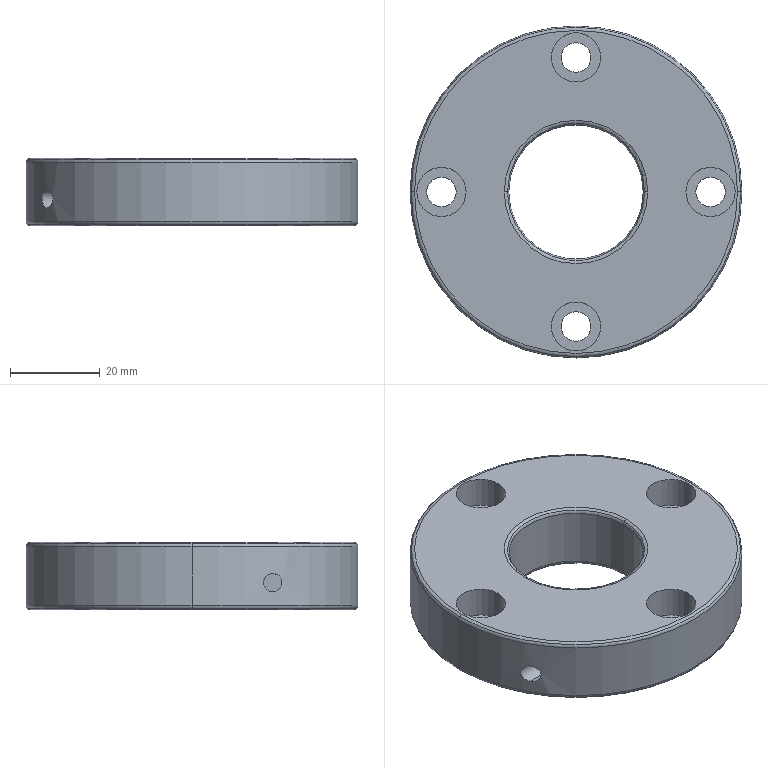Part | NX | features BREP 1 | 1 solid | 45 faces | box 74 x 74 x 15 mm | volume 49782 mm3 | cylinder 22 | torus 16 | plane 7 | commonest cylinder face diameters 6.6 x8 11 x8 4.134 x2 30 x2 74 x2
STEP:
#1=CARTESIAN_POINT('',(36.,0.,-15.));
#2=VERTEX_POINT('',#1);
#3=CARTESIAN_POINT('',(-36.,0.,-15.));
#4=VERTEX_POINT('',#3);
#5=CARTESIAN_POINT('',(0.,0.,-15.));
#6=DIRECTION('',(0.,0.,-1.));
#7=DIRECTION('',(1.,0.,0.));
#8=AXIS2_PLACEMENT_3D('',#5,#6,#7);
#9=CIRCLE('',#8,36.);
#10=EDGE_CURVE('',#2,#4,#9,.T.);
#11=ORIENTED_EDGE('',*,*,#10,.T.);
#12=CARTESIAN_POINT('',(0.,0.,-15.));
#13=DIRECTION('',(0.,0.,-1.));
#14=DIRECTION('',(-1.,0.,0.));
#15=AXIS2_PLACEMENT_3D('',#12,#13,#14);
#16=CIRCLE('',#15,36.);
#17=EDGE_CURVE('',#4,#2,#16,.T.);
#18=ORIENTED_EDGE('',*,*,#17,.T.);
#19=EDGE_LOOP('',(#11,#18));
#20=FACE_BOUND('',#19,.T.);
#21=CARTESIAN_POINT('',(3.3,30.,-15.));
#22=VERTEX_POINT('',#21);
#23=CARTESIAN_POINT('',(-3.3,30.,-15.));
#24=VERTEX_POINT('',#23);
#25=CARTESIAN_POINT('',(0.,30.,-15.));
#26=DIRECTION('',(0.,0.,1.));
#27=DIRECTION('',(1.,0.,0.));
#28=AXIS2_PLACEMENT_3D('',#25,#26,#27);
#29=CIRCLE('',#28,3.3);
#30=EDGE_CURVE('',#22,#24,#29,.T.);
#31=ORIENTED_EDGE('',*,*,#30,.T.);
#32=CARTESIAN_POINT('',(0.,30.,-15.));
#33=DIRECTION('',(0.,0.,1.));
#34=DIRECTION('',(-1.,0.,0.));
#35=AXIS2_PLACEMENT_3D('',#32,#33,#34);
#36=CIRCLE('',#35,3.3);
#37=EDGE_CURVE('',#24,#22,#36,.T.);
#38=ORIENTED_EDGE('',*,*,#37,.T.);
#39=EDGE_LOOP('',(#31,#38));
#40=FACE_BOUND('',#39,.T.);
#41=CARTESIAN_POINT('',(-26.7,0.,-15.));
#42=VERTEX_POINT('',#41);
#43=CARTESIAN_POINT('',(-33.3,0.,-15.));
#44=VERTEX_POINT('',#43);
#45=CARTESIAN_POINT('',(-30.,0.,-15.));
#46=DIRECTION('',(0.,0.,1.));
#47=DIRECTION('',(1.,0.,0.));
#48=AXIS2_PLACEMENT_3D('',#45,#46,#47);
#49=CIRCLE('',#48,3.3);
#50=EDGE_CURVE('',#42,#44,#49,.T.);
#51=ORIENTED_EDGE('',*,*,#50,.T.);
#52=CARTESIAN_POINT('',(-30.,0.,-15.));
#53=DIRECTION('',(0.,0.,1.));
#54=DIRECTION('',(-1.,0.,0.));
#55=AXIS2_PLACEMENT_3D('',#52,#53,#54);
#56=CIRCLE('',#55,3.3);
#57=EDGE_CURVE('',#44,#42,#56,.T.);
#58=ORIENTED_EDGE('',*,*,#57,.T.);
#59=EDGE_LOOP('',(#51,#58));
#60=FACE_BOUND('',#59,.T.);
#61=CARTESIAN_POINT('',(33.3,0.,-15.));
#62=VERTEX_POINT('',#61);
#63=CARTESIAN_POINT('',(26.7,0.,-15.));
#64=VERTEX_POINT('',#63);
#65=CARTESIAN_POINT('',(30.,0.,-15.));
#66=DIRECTION('',(0.,0.,1.));
#67=DIRECTION('',(1.,0.,0.));
#68=AXIS2_PLACEMENT_3D('',#65,#66,#67);
#69=CIRCLE('',#68,3.3);
#70=EDGE_CURVE('',#62,#64,#69,.T.);
#71=ORIENTED_EDGE('',*,*,#70,.T.);
#72=CARTESIAN_POINT('',(30.,0.,-15.));
#73=DIRECTION('',(0.,0.,1.));
#74=DIRECTION('',(-1.,0.,0.));
#75=AXIS2_PLACEMENT_3D('',#72,#73,#74);
#76=CIRCLE('',#75,3.3);
#77=EDGE_CURVE('',#64,#62,#76,.T.);
#78=ORIENTED_EDGE('',*,*,#77,.T.);
#79=EDGE_LOOP('',(#71,#78));
#80=FACE_BOUND('',#79,.T.);
#81=CARTESIAN_POINT('',(-3.3,-30.,-15.));
#82=VERTEX_POINT('',#81);
#83=CARTESIAN_POINT('',(3.3,-30.,-15.));
#84=VERTEX_POINT('',#83);
#85=CARTESIAN_POINT('',(0.,-30.,-15.));
#86=DIRECTION('',(0.,0.,1.));
#87=DIRECTION('',(-1.,0.,0.));
#88=AXIS2_PLACEMENT_3D('',#85,#86,#87);
#89=CIRCLE('',#88,3.3);
#90=EDGE_CURVE('',#82,#84,#89,.T.);
#91=ORIENTED_EDGE('',*,*,#90,.T.);
#92=CARTESIAN_POINT('',(0.,-30.,-15.));
#93=DIRECTION('',(0.,0.,1.));
#94=DIRECTION('',(1.,0.,0.));
#95=AXIS2_PLACEMENT_3D('',#92,#93,#94);
#96=CIRCLE('',#95,3.3);
#97=EDGE_CURVE('',#84,#82,#96,.T.);
#98=ORIENTED_EDGE('',*,*,#97,.T.);
#99=EDGE_LOOP('',(#91,#98));
#100=FACE_BOUND('',#99,.T.);
#101=CARTESIAN_POINT('',(16.,0.,-15.));
#102=VERTEX_POINT('',#101);
#103=CARTESIAN_POINT('',(-16.,0.,-15.));
#104=VERTEX_POINT('',#103);
#105=CARTESIAN_POINT('',(0.,0.,-15.));
#106=DIRECTION('',(0.,0.,1.));
#107=DIRECTION('',(1.,0.,0.));
#108=AXIS2_PLACEMENT_3D('',#105,#106,#107);
#109=CIRCLE('',#108,16.);
#110=EDGE_CURVE('',#102,#104,#109,.T.);
#111=ORIENTED_EDGE('',*,*,#110,.T.);
#112=CARTESIAN_POINT('',(0.,0.,-15.));
#113=DIRECTION('',(0.,0.,1.));
#114=DIRECTION('',(-1.,0.,0.));
#115=AXIS2_PLACEMENT_3D('',#112,#113,#114);
#116=CIRCLE('',#115,16.);
#117=EDGE_CURVE('',#104,#102,#116,.T.);
#118=ORIENTED_EDGE('',*,*,#117,.T.);
#119=EDGE_LOOP('',(#111,#118));
#120=FACE_BOUND('',#119,.T.);
#121=CARTESIAN_POINT('',(0.,16.,-15.));
#122=DIRECTION('',(0.,0.,-1.));
#123=DIRECTION('',(0.,-1.,0.));
#124=AXIS2_PLACEMENT_3D('',#121,#122,#123);
#125=PLANE('',#124);
#126=ADVANCED_FACE('',(#20,#40,#60,#80,#100,#120),#125,.T.);
#127=CARTESIAN_POINT('',(-36.707,0.,-14.707));
#128=VERTEX_POINT('',#127);
#129=CARTESIAN_POINT('',(-36.,0.,-14.));
#130=DIRECTION('',(0.,-1.,0.));
#131=DIRECTION('',(-0.7071,0.,-0.7071));
#132=AXIS2_PLACEMENT_3D('',#129,#130,#131);
#133=CIRCLE('',#132,1.);
#134=EDGE_CURVE('',#128,#4,#133,.T.);
#135=ORIENTED_EDGE('',*,*,#134,.F.);
#136=CARTESIAN_POINT('',(36.707,0.,-14.707));
#137=VERTEX_POINT('',#136);
#138=CARTESIAN_POINT('',(0.,0.,-14.707));
#139=DIRECTION('',(0.,0.,-1.));
#140=DIRECTION('',(-1.,0.,0.));
#141=AXIS2_PLACEMENT_3D('',#138,#139,#140);
#142=CIRCLE('',#141,36.707);
#143=EDGE_CURVE('',#128,#137,#142,.T.);
#144=ORIENTED_EDGE('',*,*,#143,.T.);
#145=CARTESIAN_POINT('',(36.,0.,-14.));
#146=DIRECTION('',(0.,1.,0.));
#147=DIRECTION('',(0.7071,0.,-0.7071));
#148=AXIS2_PLACEMENT_3D('',#145,#146,#147);
#149=CIRCLE('',#148,1.);
#150=EDGE_CURVE('',#137,#2,#149,.T.);
#151=ORIENTED_EDGE('',*,*,#150,.T.);
#152=ORIENTED_EDGE('',*,*,#17,.F.);
#153=EDGE_LOOP('',(#135,#144,#151,#152));
#154=FACE_BOUND('',#153,.T.);
#155=CARTESIAN_POINT('',(0.,0.,-14.));
#156=DIRECTION('',(0.,0.,-1.));
#157=DIRECTION('',(-1.,0.,0.));
#158=AXIS2_PLACEMENT_3D('',#155,#156,#157);
#159=TOROIDAL_SURFACE('',#158,36.,1.);
#160=ADVANCED_FACE('',(#154),#159,.T.);
#161=ORIENTED_EDGE('',*,*,#150,.F.);
#162=CARTESIAN_POINT('',(0.,0.,-14.707));
#163=DIRECTION('',(0.,0.,-1.));
#164=DIRECTION('',(1.,0.,0.));
#165=AXIS2_PLACEMENT_3D('',#162,#163,#164);
#166=CIRCLE('',#165,36.707);
#167=EDGE_CURVE('',#137,#128,#166,.T.);
#168=ORIENTED_EDGE('',*,*,#167,.T.);
#169=ORIENTED_EDGE('',*,*,#134,.T.);
#170=ORIENTED_EDGE('',*,*,#10,.F.);
#171=EDGE_LOOP('',(#161,#168,#169,#170));
#172=FACE_BOUND('',#171,.T.);
#173=CARTESIAN_POINT('',(0.,0.,-14.));
#174=DIRECTION('',(0.,0.,-1.));
#175=DIRECTION('',(-1.,0.,0.));
#176=AXIS2_PLACEMENT_3D('',#173,#174,#175);
#177=TOROIDAL_SURFACE('',#176,36.,1.);
#178=ADVANCED_FACE('',(#172),#177,.T.);
#179=CARTESIAN_POINT('',(-37.,0.,-14.));
#180=VERTEX_POINT('',#179);
#181=CARTESIAN_POINT('',(-36.,0.,-14.));
#182=DIRECTION('',(0.,-1.,0.));
#183=DIRECTION('',(-1.,0.,0.));
#184=AXIS2_PLACEMENT_3D('',#181,#182,#183);
#185=CIRCLE('',#184,1.);
#186=EDGE_CURVE('',#180,#128,#185,.T.);
#187=ORIENTED_EDGE('',*,*,#186,.T.);
#188=ORIENTED_EDGE('',*,*,#167,.F.);
#189=CARTESIAN_POINT('',(37.,0.,-14.));
#190=VERTEX_POINT('',#189);
#191=CARTESIAN_POINT('',(36.,0.,-14.));
#192=DIRECTION('',(0.,1.,0.));
#193=DIRECTION('',(1.,0.,0.));
#194=AXIS2_PLACEMENT_3D('',#191,#192,#193);
#195=CIRCLE('',#194,1.);
#196=EDGE_CURVE('',#190,#137,#195,.T.);
#197=ORIENTED_EDGE('',*,*,#196,.F.);
#198=CARTESIAN_POINT('',(0.,0.,-14.));
#199=DIRECTION('',(0.,0.,-1.));
#200=DIRECTION('',(1.,0.,0.));
#201=AXIS2_PLACEMENT_3D('',#198,#199,#200);
#202=CIRCLE('',#201,37.);
#203=EDGE_CURVE('',#190,#180,#202,.T.);
#204=ORIENTED_EDGE('',*,*,#203,.T.);
#205=EDGE_LOOP('',(#187,#188,#197,#204));
#206=FACE_BOUND('',#205,.T.);
#207=CARTESIAN_POINT('',(0.,0.,-14.));
#208=DIRECTION('',(0.,0.,-1.));
#209=DIRECTION('',(-1.,0.,0.));
#210=AXIS2_PLACEMENT_3D('',#207,#208,#209);
#211=TOROIDAL_SURFACE('',#210,36.,1.);
#212=ADVANCED_FACE('',(#206),#211,.T.);
#213=CARTESIAN_POINT('',(37.,0.,-1.));
#214=VERTEX_POINT('',#213);
#215=CARTESIAN_POINT('',(37.,0.,-14.));
#216=DIRECTION('',(0.,0.,1.));
#217=VECTOR('',#216,1000.);
#218=LINE('',#215,#217);
#219=EDGE_CURVE('',#214,#190,#218,.F.);
#220=ORIENTED_EDGE('',*,*,#219,.F.);
#221=CARTESIAN_POINT('',(-37.,0.,-1.));
#222=VERTEX_POINT('',#221);
#223=CARTESIAN_POINT('',(0.,0.,-1.));
#224=DIRECTION('',(0.,0.,1.));
#225=DIRECTION('',(-1.,0.,0.));
#226=AXIS2_PLACEMENT_3D('',#223,#224,#225);
#227=CIRCLE('',#226,37.);
#228=EDGE_CURVE('',#222,#214,#227,.T.);
#229=ORIENTED_EDGE('',*,*,#228,.F.);
#230=CARTESIAN_POINT('',(-37.,0.,-14.));
#231=DIRECTION('',(0.,0.,1.));
#232=VECTOR('',#231,1000.);
#233=LINE('',#230,#232);
#234=EDGE_CURVE('',#222,#180,#233,.F.);
#235=ORIENTED_EDGE('',*,*,#234,.T.);
#236=ORIENTED_EDGE('',*,*,#203,.F.);
#237=EDGE_LOOP('',(#220,#229,#235,#236));
#238=FACE_BOUND('',#237,.T.);
#239=CARTESIAN_POINT('',(-32.326,-18.,-11.067));
#240=VERTEX_POINT('',#239);
#241=CARTESIAN_POINT('',(-32.294,-18.057,-11.066));
#242=VERTEX_POINT('',#241);
#243=CARTESIAN_POINT('',(-32.326,-18.,-11.067));
#244=CARTESIAN_POINT('',(-32.323,-18.006,-11.067));
#245=CARTESIAN_POINT('',(-32.316,-18.019,-11.067));
#246=CARTESIAN_POINT('',(-32.305,-18.038,-11.067));
#247=CARTESIAN_POINT('',(-32.298,-18.051,-11.066));
#248=CARTESIAN_POINT('',(-32.294,-18.057,-11.066));
#249=B_SPLINE_CURVE_WITH_KNOTS('',3,(#243,#244,#245,#246,#247,#248),.UNSPECIFIED.,.F.,.F.,(4,1,1,4),(0.,0.3333,0.6667,1.),.UNSPECIFIED.);
#250=EDGE_CURVE('',#240,#242,#249,.T.);
#251=ORIENTED_EDGE('',*,*,#250,.F.);
#252=CARTESIAN_POINT('',(-32.326,-18.,-6.933));
#253=VERTEX_POINT('',#252);
#254=CARTESIAN_POINT('',(-32.326,-18.,-11.067));
#255=CARTESIAN_POINT('',(-32.651,-17.416,-11.067));
#256=CARTESIAN_POINT('',(-33.218,-16.314,-10.542));
#257=CARTESIAN_POINT('',(-33.483,-15.741,-8.996));
#258=CARTESIAN_POINT('',(-33.214,-16.322,-7.45));
#259=CARTESIAN_POINT('',(-32.649,-17.421,-6.933));
#260=CARTESIAN_POINT('',(-32.326,-18.,-6.933));
#261=B_SPLINE_CURVE_WITH_KNOTS('',3,(#254,#255,#256,#257,#258,#259,#260),.UNSPECIFIED.,.F.,.F.,(4,1,1,1,4),(0.,0.25,0.5,0.75,1.),.UNSPECIFIED.);
#262=EDGE_CURVE('',#253,#240,#261,.F.);
#263=ORIENTED_EDGE('',*,*,#262,.F.);
#264=CARTESIAN_POINT('',(-32.326,-18.,-6.933));
#265=CARTESIAN_POINT('',(-32.002,-18.582,-6.933));
#266=CARTESIAN_POINT('',(-31.326,-19.706,-7.48));
#267=CARTESIAN_POINT('',(-30.97,-20.241,-8.978));
#268=CARTESIAN_POINT('',(-31.308,-19.733,-10.483));
#269=CARTESIAN_POINT('',(-31.969,-18.639,-11.05));
#270=CARTESIAN_POINT('',(-32.294,-18.057,-11.066));
#271=B_SPLINE_CURVE_WITH_KNOTS('',3,(#264,#265,#266,#267,#268,#269,#270),.UNSPECIFIED.,.F.,.F.,(4,1,1,1,4),(0.,0.25,0.5,0.75,1.),.UNSPECIFIED.);
#272=EDGE_CURVE('',#242,#253,#271,.F.);
#273=ORIENTED_EDGE('',*,*,#272,.F.);
#274=EDGE_LOOP('',(#251,#263,#273));
#275=FACE_BOUND('',#274,.T.);
#276=CARTESIAN_POINT('',(0.,0.,-50.));
#277=DIRECTION('',(0.,0.,1.));
#278=DIRECTION('',(-1.,0.,0.));
#279=AXIS2_PLACEMENT_3D('',#276,#277,#278);
#280=CYLINDRICAL_SURFACE('',#279,37.);
#281=ADVANCED_FACE('',(#238,#275),#280,.T.);
#282=ORIENTED_EDGE('',*,*,#234,.F.);
#283=CARTESIAN_POINT('',(0.,0.,-1.));
#284=DIRECTION('',(0.,0.,1.));
#285=DIRECTION('',(1.,0.,0.));
#286=AXIS2_PLACEMENT_3D('',#283,#284,#285);
#287=CIRCLE('',#286,37.);
#288=EDGE_CURVE('',#214,#222,#287,.T.);
#289=ORIENTED_EDGE('',*,*,#288,.F.);
#290=ORIENTED_EDGE('',*,*,#219,.T.);
#291=CARTESIAN_POINT('',(0.,0.,-14.));
#292=DIRECTION('',(0.,0.,-1.));
#293=DIRECTION('',(-1.,0.,0.));
#294=AXIS2_PLACEMENT_3D('',#291,#292,#293);
#295=CIRCLE('',#294,37.);
#296=EDGE_CURVE('',#180,#190,#295,.T.);
#297=ORIENTED_EDGE('',*,*,#296,.F.);
#298=EDGE_LOOP('',(#282,#289,#290,#297));
#299=FACE_BOUND('',#298,.T.);
#300=CARTESIAN_POINT('',(0.,0.,-50.));
#301=DIRECTION('',(0.,0.,1.));
#302=DIRECTION('',(-1.,0.,0.));
#303=AXIS2_PLACEMENT_3D('',#300,#301,#302);
#304=CYLINDRICAL_SURFACE('',#303,37.);
#305=ADVANCED_FACE('',(#299),#304,.T.);
#306=ORIENTED_EDGE('',*,*,#196,.T.);
#307=ORIENTED_EDGE('',*,*,#143,.F.);
#308=ORIENTED_EDGE('',*,*,#186,.F.);
#309=ORIENTED_EDGE('',*,*,#296,.T.);
#310=EDGE_LOOP('',(#306,#307,#308,#309));
#311=FACE_BOUND('',#310,.T.);
#312=CARTESIAN_POINT('',(0.,0.,-14.));
#313=DIRECTION('',(0.,0.,-1.));
#314=DIRECTION('',(-1.,0.,0.));
#315=AXIS2_PLACEMENT_3D('',#312,#313,#314);
#316=TOROIDAL_SURFACE('',#315,36.,1.);
#317=ADVANCED_FACE('',(#311),#316,.T.);
#318=CARTESIAN_POINT('',(-36.707,0.,-0.2929));
#319=VERTEX_POINT('',#318);
#320=CARTESIAN_POINT('',(-36.,0.,-1.));
#321=DIRECTION('',(0.,-1.,0.));
#322=DIRECTION('',(-0.7071,0.,0.7071));
#323=AXIS2_PLACEMENT_3D('',#320,#321,#322);
#324=CIRCLE('',#323,1.);
#325=EDGE_CURVE('',#319,#222,#324,.T.);
#326=ORIENTED_EDGE('',*,*,#325,.F.);
#327=CARTESIAN_POINT('',(36.707,0.,-0.2929));
#328=VERTEX_POINT('',#327);
#329=CARTESIAN_POINT('',(0.,0.,-0.2929));
#330=DIRECTION('',(0.,0.,-1.));
#331=DIRECTION('',(-1.,0.,0.));
#332=AXIS2_PLACEMENT_3D('',#329,#330,#331);
#333=CIRCLE('',#332,36.707);
#334=EDGE_CURVE('',#319,#328,#333,.T.);
#335=ORIENTED_EDGE('',*,*,#334,.T.);
#336=CARTESIAN_POINT('',(36.,0.,-1.));
#337=DIRECTION('',(0.,1.,0.));
#338=DIRECTION('',(0.7071,0.,0.7071));
#339=AXIS2_PLACEMENT_3D('',#336,#337,#338);
#340=CIRCLE('',#339,1.);
#341=EDGE_CURVE('',#328,#214,#340,.T.);
#342=ORIENTED_EDGE('',*,*,#341,.T.);
#343=ORIENTED_EDGE('',*,*,#288,.T.);
#344=EDGE_LOOP('',(#326,#335,#342,#343));
#345=FACE_BOUND('',#344,.T.);
#346=CARTESIAN_POINT('',(0.,0.,-1.));
#347=DIRECTION('',(0.,0.,-1.));
#348=DIRECTION('',(-1.,0.,0.));
#349=AXIS2_PLACEMENT_3D('',#346,#347,#348);
#350=TOROIDAL_SURFACE('',#349,36.,1.);
#351=ADVANCED_FACE('',(#345),#350,.T.);
#352=ORIENTED_EDGE('',*,*,#341,.F.);
#353=CARTESIAN_POINT('',(0.,0.,-0.2929));
#354=DIRECTION('',(0.,0.,-1.));
#355=DIRECTION('',(1.,0.,0.));
#356=AXIS2_PLACEMENT_3D('',#353,#354,#355);
#357=CIRCLE('',#356,36.707);
#358=EDGE_CURVE('',#328,#319,#357,.T.);
#359=ORIENTED_EDGE('',*,*,#358,.T.);
#360=ORIENTED_EDGE('',*,*,#325,.T.);
#361=ORIENTED_EDGE('',*,*,#228,.T.);
#362=EDGE_LOOP('',(#352,#359,#360,#361));
#363=FACE_BOUND('',#362,.T.);
#364=CARTESIAN_POINT('',(0.,0.,-1.));
#365=DIRECTION('',(0.,0.,-1.));
#366=DIRECTION('',(-1.,0.,0.));
#367=AXIS2_PLACEMENT_3D('',#364,#365,#366);
#368=TOROIDAL_SURFACE('',#367,36.,1.);
#369=ADVANCED_FACE('',(#363),#368,.T.);
#370=CARTESIAN_POINT('',(-36.,0.,0.));
#371=VERTEX_POINT('',#370);
#372=CARTESIAN_POINT('',(-36.,0.,-1.));
#373=DIRECTION('',(0.,-1.,0.));
#374=DIRECTION('',(0.,0.,1.));
#375=AXIS2_PLACEMENT_3D('',#372,#373,#374);
#376=CIRCLE('',#375,1.);
#377=EDGE_CURVE('',#371,#319,#376,.T.);
#378=ORIENTED_EDGE('',*,*,#377,.T.);
#379=ORIENTED_EDGE('',*,*,#358,.F.);
#380=CARTESIAN_POINT('',(36.,0.,0.));
#381=VERTEX_POINT('',#380);
#382=CARTESIAN_POINT('',(36.,0.,-1.));
#383=DIRECTION('',(0.,1.,0.));
#384=DIRECTION('',(0.,0.,1.));
#385=AXIS2_PLACEMENT_3D('',#382,#383,#384);
#386=CIRCLE('',#385,1.);
#387=EDGE_CURVE('',#381,#328,#386,.T.);
#388=ORIENTED_EDGE('',*,*,#387,.F.);
#389=CARTESIAN_POINT('',(0.,0.,0.));
#390=DIRECTION('',(0.,0.,1.));
#391=DIRECTION('',(-1.,0.,0.));
#392=AXIS2_PLACEMENT_3D('',#389,#390,#391);
#393=CIRCLE('',#392,36.);
#394=EDGE_CURVE('',#371,#381,#393,.T.);
#395=ORIENTED_EDGE('',*,*,#394,.F.);
#396=EDGE_LOOP('',(#378,#379,#388,#395));
#397=FACE_BOUND('',#396,.T.);
#398=CARTESIAN_POINT('',(0.,0.,-1.));
#399=DIRECTION('',(0.,0.,-1.));
#400=DIRECTION('',(-1.,0.,0.));
#401=AXIS2_PLACEMENT_3D('',#398,#399,#400);
#402=TOROIDAL_SURFACE('',#401,36.,1.);
#403=ADVANCED_FACE('',(#397),#402,.T.);
#404=CARTESIAN_POINT('',(0.,0.,0.));
#405=DIRECTION('',(0.,0.,1.));
#406=DIRECTION('',(1.,0.,0.));
#407=AXIS2_PLACEMENT_3D('',#404,#405,#406);
#408=CIRCLE('',#407,36.);
#409=EDGE_CURVE('',#381,#371,#408,.T.);
#410=ORIENTED_EDGE('',*,*,#409,.T.);
#411=ORIENTED_EDGE('',*,*,#394,.T.);
#412=EDGE_LOOP('',(#410,#411));
#413=FACE_BOUND('',#412,.T.);
#414=CARTESIAN_POINT('',(16.,0.,0.));
#415=VERTEX_POINT('',#414);
#416=CARTESIAN_POINT('',(-16.,0.,0.));
#417=VERTEX_POINT('',#416);
#418=CARTESIAN_POINT('',(0.,0.,0.));
#419=DIRECTION('',(0.,0.,-1.));
#420=DIRECTION('',(1.,0.,0.));
#421=AXIS2_PLACEMENT_3D('',#418,#419,#420);
#422=CIRCLE('',#421,16.);
#423=EDGE_CURVE('',#415,#417,#422,.T.);
#424=ORIENTED_EDGE('',*,*,#423,.T.);
#425=CARTESIAN_POINT('',(0.,0.,0.));
#426=DIRECTION('',(0.,0.,-1.));
#427=DIRECTION('',(-1.,0.,0.));
#428=AXIS2_PLACEMENT_3D('',#425,#426,#427);
#429=CIRCLE('',#428,16.);
#430=EDGE_CURVE('',#417,#415,#429,.T.);
#431=ORIENTED_EDGE('',*,*,#430,.T.);
#432=EDGE_LOOP('',(#424,#431));
#433=FACE_BOUND('',#432,.T.);
#434=CARTESIAN_POINT('',(-5.5,30.,0.));
#435=VERTEX_POINT('',#434);
#436=CARTESIAN_POINT('',(5.5,30.,0.));
#437=VERTEX_POINT('',#436);
#438=CARTESIAN_POINT('',(0.,30.,0.));
#439=DIRECTION('',(0.,0.,-1.));
#440=DIRECTION('',(-1.,0.,0.));
#441=AXIS2_PLACEMENT_3D('',#438,#439,#440);
#442=CIRCLE('',#441,5.5);
#443=EDGE_CURVE('',#435,#437,#442,.T.);
#444=ORIENTED_EDGE('',*,*,#443,.T.);
#445=CARTESIAN_POINT('',(0.,30.,0.));
#446=DIRECTION('',(0.,0.,-1.));
#447=DIRECTION('',(1.,0.,0.));
#448=AXIS2_PLACEMENT_3D('',#445,#446,#447);
#449=CIRCLE('',#448,5.5);
#450=EDGE_CURVE('',#437,#435,#449,.T.);
#451=ORIENTED_EDGE('',*,*,#450,.T.);
#452=EDGE_LOOP('',(#444,#451));
#453=FACE_BOUND('',#452,.T.);
#454=CARTESIAN_POINT('',(-24.5,0.,0.));
#455=VERTEX_POINT('',#454);
#456=CARTESIAN_POINT('',(-35.5,0.,0.));
#457=VERTEX_POINT('',#456);
#458=CARTESIAN_POINT('',(-30.,0.,0.));
#459=DIRECTION('',(0.,0.,-1.));
#460=DIRECTION('',(1.,0.,0.));
#461=AXIS2_PLACEMENT_3D('',#458,#459,#460);
#462=CIRCLE('',#461,5.5);
#463=EDGE_CURVE('',#455,#457,#462,.T.);
#464=ORIENTED_EDGE('',*,*,#463,.T.);
#465=CARTESIAN_POINT('',(-30.,0.,0.));
#466=DIRECTION('',(0.,0.,-1.));
#467=DIRECTION('',(-1.,0.,0.));
#468=AXIS2_PLACEMENT_3D('',#465,#466,#467);
#469=CIRCLE('',#468,5.5);
#470=EDGE_CURVE('',#457,#455,#469,.T.);
#471=ORIENTED_EDGE('',*,*,#470,.T.);
#472=EDGE_LOOP('',(#464,#471));
#473=FACE_BOUND('',#472,.T.);
#474=CARTESIAN_POINT('',(35.5,0.,0.));
#475=VERTEX_POINT('',#474);
#476=CARTESIAN_POINT('',(24.5,0.,0.));
#477=VERTEX_POINT('',#476);
#478=CARTESIAN_POINT('',(30.,0.,0.));
#479=DIRECTION('',(0.,0.,-1.));
#480=DIRECTION('',(1.,0.,0.));
#481=AXIS2_PLACEMENT_3D('',#478,#479,#480);
#482=CIRCLE('',#481,5.5);
#483=EDGE_CURVE('',#475,#477,#482,.T.);
#484=ORIENTED_EDGE('',*,*,#483,.T.);
#485=CARTESIAN_POINT('',(30.,0.,0.));
#486=DIRECTION('',(0.,0.,-1.));
#487=DIRECTION('',(-1.,0.,0.));
#488=AXIS2_PLACEMENT_3D('',#485,#486,#487);
#489=CIRCLE('',#488,5.5);
#490=EDGE_CURVE('',#477,#475,#489,.T.);
#491=ORIENTED_EDGE('',*,*,#490,.T.);
#492=EDGE_LOOP('',(#484,#491));
#493=FACE_BOUND('',#492,.T.);
#494=CARTESIAN_POINT('',(-5.5,-30.,0.));
#495=VERTEX_POINT('',#494);
#496=CARTESIAN_POINT('',(5.5,-30.,0.));
#497=VERTEX_POINT('',#496);
#498=CARTESIAN_POINT('',(0.,-30.,0.));
#499=DIRECTION('',(0.,0.,-1.));
#500=DIRECTION('',(-1.,0.,0.));
#501=AXIS2_PLACEMENT_3D('',#498,#499,#500);
#502=CIRCLE('',#501,5.5);
#503=EDGE_CURVE('',#495,#497,#502,.T.);
#504=ORIENTED_EDGE('',*,*,#503,.T.);
#505=CARTESIAN_POINT('',(0.,-30.,0.));
#506=DIRECTION('',(0.,0.,-1.));
#507=DIRECTION('',(1.,0.,0.));
#508=AXIS2_PLACEMENT_3D('',#505,#506,#507);
#509=CIRCLE('',#508,5.5);
#510=EDGE_CURVE('',#497,#495,#509,.T.);
#511=ORIENTED_EDGE('',*,*,#510,.T.);
#512=EDGE_LOOP('',(#504,#511));
#513=FACE_BOUND('',#512,.T.);
#514=CARTESIAN_POINT('',(0.,36.,0.));
#515=DIRECTION('',(0.,0.,1.));
#516=DIRECTION('',(1.,0.,0.));
#517=AXIS2_PLACEMENT_3D('',#514,#515,#516);
#518=PLANE('',#517);
#519=ADVANCED_FACE('',(#413,#433,#453,#473,#493,#513),#518,.T.);
#520=ORIENTED_EDGE('',*,*,#387,.T.);
#521=ORIENTED_EDGE('',*,*,#334,.F.);
#522=ORIENTED_EDGE('',*,*,#377,.F.);
#523=ORIENTED_EDGE('',*,*,#409,.F.);
#524=EDGE_LOOP('',(#520,#521,#522,#523));
#525=FACE_BOUND('',#524,.T.);
#526=CARTESIAN_POINT('',(0.,0.,-1.));
#527=DIRECTION('',(0.,0.,-1.));
#528=DIRECTION('',(-1.,0.,0.));
#529=AXIS2_PLACEMENT_3D('',#526,#527,#528);
#530=TOROIDAL_SURFACE('',#529,36.,1.);
#531=ADVANCED_FACE('',(#525),#530,.T.);
#532=CARTESIAN_POINT('',(-15.293,0.,-0.2929));
#533=VERTEX_POINT('',#532);
#534=CARTESIAN_POINT('',(-16.,0.,-1.));
#535=DIRECTION('',(0.,-1.,0.));
#536=DIRECTION('',(0.7071,0.,0.7071));
#537=AXIS2_PLACEMENT_3D('',#534,#535,#536);
#538=CIRCLE('',#537,1.);
#539=EDGE_CURVE('',#533,#417,#538,.T.);
#540=ORIENTED_EDGE('',*,*,#539,.F.);
#541=CARTESIAN_POINT('',(15.293,0.,-0.2929));
#542=VERTEX_POINT('',#541);
#543=CARTESIAN_POINT('',(0.,0.,-0.2929));
#544=DIRECTION('',(0.,0.,-1.));
#545=DIRECTION('',(-1.,0.,0.));
#546=AXIS2_PLACEMENT_3D('',#543,#544,#545);
#547=CIRCLE('',#546,15.293);
#548=EDGE_CURVE('',#533,#542,#547,.T.);
#549=ORIENTED_EDGE('',*,*,#548,.T.);
#550=CARTESIAN_POINT('',(16.,0.,-1.));
#551=DIRECTION('',(0.,1.,0.));
#552=DIRECTION('',(-0.7071,0.,0.7071));
#553=AXIS2_PLACEMENT_3D('',#550,#551,#552);
#554=CIRCLE('',#553,1.);
#555=EDGE_CURVE('',#542,#415,#554,.T.);
#556=ORIENTED_EDGE('',*,*,#555,.T.);
#557=ORIENTED_EDGE('',*,*,#430,.F.);
#558=EDGE_LOOP('',(#540,#549,#556,#557));
#559=FACE_BOUND('',#558,.T.);
#560=CARTESIAN_POINT('',(0.,0.,-1.));
#561=DIRECTION('',(0.,0.,-1.));
#562=DIRECTION('',(-1.,0.,0.));
#563=AXIS2_PLACEMENT_3D('',#560,#561,#562);
#564=TOROIDAL_SURFACE('',#563,16.,1.);
#565=ADVANCED_FACE('',(#559),#564,.T.);
#566=ORIENTED_EDGE('',*,*,#555,.F.);
#567=CARTESIAN_POINT('',(0.,0.,-0.2929));
#568=DIRECTION('',(0.,0.,-1.));
#569=DIRECTION('',(1.,0.,0.));
#570=AXIS2_PLACEMENT_3D('',#567,#568,#569);
#571=CIRCLE('',#570,15.293);
#572=EDGE_CURVE('',#542,#533,#571,.T.);
#573=ORIENTED_EDGE('',*,*,#572,.T.);
#574=ORIENTED_EDGE('',*,*,#539,.T.);
#575=ORIENTED_EDGE('',*,*,#423,.F.);
#576=EDGE_LOOP('',(#566,#573,#574,#575));
#577=FACE_BOUND('',#576,.T.);
#578=CARTESIAN_POINT('',(0.,0.,-1.));
#579=DIRECTION('',(0.,0.,-1.));
#580=DIRECTION('',(-1.,0.,0.));
#581=AXIS2_PLACEMENT_3D('',#578,#579,#580);
#582=TOROIDAL_SURFACE('',#581,16.,1.);
#583=ADVANCED_FACE('',(#577),#582,.T.);
#584=CARTESIAN_POINT('',(-15.,0.,-1.));
#585=VERTEX_POINT('',#584);
#586=CARTESIAN_POINT('',(-16.,0.,-1.));
#587=DIRECTION('',(0.,-1.,0.));
#588=DIRECTION('',(1.,0.,0.));
#589=AXIS2_PLACEMENT_3D('',#586,#587,#588);
#590=CIRCLE('',#589,1.);
#591=EDGE_CURVE('',#585,#533,#590,.T.);
#592=ORIENTED_EDGE('',*,*,#591,.T.);
#593=ORIENTED_EDGE('',*,*,#572,.F.);
#594=CARTESIAN_POINT('',(15.,0.,-1.));
#595=VERTEX_POINT('',#594);
#596=CARTESIAN_POINT('',(16.,0.,-1.));
#597=DIRECTION('',(0.,1.,0.));
#598=DIRECTION('',(-1.,0.,0.));
#599=AXIS2_PLACEMENT_3D('',#596,#597,#598);
#600=CIRCLE('',#599,1.);
#601=EDGE_CURVE('',#595,#542,#600,.T.);
#602=ORIENTED_EDGE('',*,*,#601,.F.);
#603=CARTESIAN_POINT('',(0.,0.,-1.));
#604=DIRECTION('',(0.,0.,-1.));
#605=DIRECTION('',(1.,0.,0.));
#606=AXIS2_PLACEMENT_3D('',#603,#604,#605);
#607=CIRCLE('',#606,15.);
#608=EDGE_CURVE('',#595,#585,#607,.T.);
#609=ORIENTED_EDGE('',*,*,#608,.T.);
#610=EDGE_LOOP('',(#592,#593,#602,#609));
#611=FACE_BOUND('',#610,.T.);
#612=CARTESIAN_POINT('',(0.,0.,-1.));
#613=DIRECTION('',(0.,0.,-1.));
#614=DIRECTION('',(-1.,0.,0.));
#615=AXIS2_PLACEMENT_3D('',#612,#613,#614);
#616=TOROIDAL_SURFACE('',#615,16.,1.);
#617=ADVANCED_FACE('',(#611),#616,.T.);
#618=CARTESIAN_POINT('',(15.,0.,-14.));
#619=VERTEX_POINT('',#618);
#620=CARTESIAN_POINT('',(15.,0.,-14.));
#621=DIRECTION('',(0.,0.,1.));
#622=VECTOR('',#621,1000.);
#623=LINE('',#620,#622);
#624=EDGE_CURVE('',#595,#619,#623,.F.);
#625=ORIENTED_EDGE('',*,*,#624,.T.);
#626=CARTESIAN_POINT('',(-15.,0.,-14.));
#627=VERTEX_POINT('',#626);
#628=CARTESIAN_POINT('',(0.,0.,-14.));
#629=DIRECTION('',(0.,0.,1.));
#630=DIRECTION('',(-1.,0.,0.));
#631=AXIS2_PLACEMENT_3D('',#628,#629,#630);
#632=CIRCLE('',#631,15.);
#633=EDGE_CURVE('',#627,#619,#632,.T.);
#634=ORIENTED_EDGE('',*,*,#633,.F.);
#635=CARTESIAN_POINT('',(-15.,0.,-14.));
#636=DIRECTION('',(0.,0.,1.));
#637=VECTOR('',#636,1000.);
#638=LINE('',#635,#637);
#639=EDGE_CURVE('',#585,#627,#638,.F.);
#640=ORIENTED_EDGE('',*,*,#639,.F.);
#641=ORIENTED_EDGE('',*,*,#608,.F.);
#642=EDGE_LOOP('',(#625,#634,#640,#641));
#643=FACE_BOUND('',#642,.T.);
#644=CARTESIAN_POINT('',(0.,0.,-50.));
#645=DIRECTION('',(0.,0.,1.));
#646=DIRECTION('',(-1.,0.,0.));
#647=AXIS2_PLACEMENT_3D('',#644,#645,#646);
#648=CYLINDRICAL_SURFACE('',#647,15.);
#649=ADVANCED_FACE('',(#643),#648,.F.);
#650=ORIENTED_EDGE('',*,*,#639,.T.);
#651=CARTESIAN_POINT('',(0.,0.,-14.));
#652=DIRECTION('',(0.,0.,1.));
#653=DIRECTION('',(1.,0.,0.));
#654=AXIS2_PLACEMENT_3D('',#651,#652,#653);
#655=CIRCLE('',#654,15.);
#656=EDGE_CURVE('',#619,#627,#655,.T.);
#657=ORIENTED_EDGE('',*,*,#656,.F.);
#658=ORIENTED_EDGE('',*,*,#624,.F.);
#659=CARTESIAN_POINT('',(0.,0.,-1.));
#660=DIRECTION('',(0.,0.,-1.));
#661=DIRECTION('',(-1.,0.,0.));
#662=AXIS2_PLACEMENT_3D('',#659,#660,#661);
#663=CIRCLE('',#662,15.);
#664=EDGE_CURVE('',#585,#595,#663,.T.);
#665=ORIENTED_EDGE('',*,*,#664,.F.);
#666=EDGE_LOOP('',(#650,#657,#658,#665));
#667=FACE_BOUND('',#666,.T.);
#668=CARTESIAN_POINT('',(0.,0.,-50.));
#669=DIRECTION('',(0.,0.,1.));
#670=DIRECTION('',(-1.,0.,0.));
#671=AXIS2_PLACEMENT_3D('',#668,#669,#670);
#672=CYLINDRICAL_SURFACE('',#671,15.);
#673=ADVANCED_FACE('',(#667),#672,.F.);
#674=ORIENTED_EDGE('',*,*,#601,.T.);
#675=ORIENTED_EDGE('',*,*,#548,.F.);
#676=ORIENTED_EDGE('',*,*,#591,.F.);
#677=ORIENTED_EDGE('',*,*,#664,.T.);
#678=EDGE_LOOP('',(#674,#675,#676,#677));
#679=FACE_BOUND('',#678,.T.);
#680=CARTESIAN_POINT('',(0.,0.,-1.));
#681=DIRECTION('',(0.,0.,-1.));
#682=DIRECTION('',(-1.,0.,0.));
#683=AXIS2_PLACEMENT_3D('',#680,#681,#682);
#684=TOROIDAL_SURFACE('',#683,16.,1.);
#685=ADVANCED_FACE('',(#679),#684,.T.);
#686=CARTESIAN_POINT('',(-15.293,0.,-14.707));
#687=VERTEX_POINT('',#686);
#688=CARTESIAN_POINT('',(-16.,0.,-14.));
#689=DIRECTION('',(0.,-1.,0.));
#690=DIRECTION('',(0.7071,0.,-0.7071));
#691=AXIS2_PLACEMENT_3D('',#688,#689,#690);
#692=CIRCLE('',#691,1.);
#693=EDGE_CURVE('',#687,#627,#692,.T.);
#694=ORIENTED_EDGE('',*,*,#693,.F.);
#695=CARTESIAN_POINT('',(15.293,0.,-14.707));
#696=VERTEX_POINT('',#695);
#697=CARTESIAN_POINT('',(0.,0.,-14.707));
#698=DIRECTION('',(0.,0.,-1.));
#699=DIRECTION('',(-1.,0.,0.));
#700=AXIS2_PLACEMENT_3D('',#697,#698,#699);
#701=CIRCLE('',#700,15.293);
#702=EDGE_CURVE('',#687,#696,#701,.T.);
#703=ORIENTED_EDGE('',*,*,#702,.T.);
#704=CARTESIAN_POINT('',(16.,0.,-14.));
#705=DIRECTION('',(0.,1.,0.));
#706=DIRECTION('',(-0.7071,0.,-0.7071));
#707=AXIS2_PLACEMENT_3D('',#704,#705,#706);
#708=CIRCLE('',#707,1.);
#709=EDGE_CURVE('',#696,#619,#708,.T.);
#710=ORIENTED_EDGE('',*,*,#709,.T.);
#711=ORIENTED_EDGE('',*,*,#656,.T.);
#712=EDGE_LOOP('',(#694,#703,#710,#711));
#713=FACE_BOUND('',#712,.T.);
#714=CARTESIAN_POINT('',(0.,0.,-14.));
#715=DIRECTION('',(0.,0.,-1.));
#716=DIRECTION('',(-1.,0.,0.));
#717=AXIS2_PLACEMENT_3D('',#714,#715,#716);
#718=TOROIDAL_SURFACE('',#717,16.,1.);
#719=ADVANCED_FACE('',(#713),#718,.T.);
#720=ORIENTED_EDGE('',*,*,#709,.F.);
#721=CARTESIAN_POINT('',(0.,0.,-14.707));
#722=DIRECTION('',(0.,0.,-1.));
#723=DIRECTION('',(1.,0.,0.));
#724=AXIS2_PLACEMENT_3D('',#721,#722,#723);
#725=CIRCLE('',#724,15.293);
#726=EDGE_CURVE('',#696,#687,#725,.T.);
#727=ORIENTED_EDGE('',*,*,#726,.T.);
#728=ORIENTED_EDGE('',*,*,#693,.T.);
#729=ORIENTED_EDGE('',*,*,#633,.T.);
#730=EDGE_LOOP('',(#720,#727,#728,#729));
#731=FACE_BOUND('',#730,.T.);
#732=CARTESIAN_POINT('',(0.,0.,-14.));
#733=DIRECTION('',(0.,0.,-1.));
#734=DIRECTION('',(-1.,0.,0.));
#735=AXIS2_PLACEMENT_3D('',#732,#733,#734);
#736=TOROIDAL_SURFACE('',#735,16.,1.);
#737=ADVANCED_FACE('',(#731),#736,.T.);
#738=CARTESIAN_POINT('',(-16.,0.,-14.));
#739=DIRECTION('',(0.,-1.,0.));
#740=DIRECTION('',(0.,0.,-1.));
#741=AXIS2_PLACEMENT_3D('',#738,#739,#740);
#742=CIRCLE('',#741,1.);
#743=EDGE_CURVE('',#104,#687,#742,.T.);
#744=ORIENTED_EDGE('',*,*,#743,.T.);
#745=ORIENTED_EDGE('',*,*,#726,.F.);
#746=CARTESIAN_POINT('',(16.,0.,-14.));
#747=DIRECTION('',(0.,1.,0.));
#748=DIRECTION('',(0.,0.,-1.));
#749=AXIS2_PLACEMENT_3D('',#746,#747,#748);
#750=CIRCLE('',#749,1.);
#751=EDGE_CURVE('',#102,#696,#750,.T.);
#752=ORIENTED_EDGE('',*,*,#751,.F.);
#753=ORIENTED_EDGE('',*,*,#117,.F.);
#754=EDGE_LOOP('',(#744,#745,#752,#753));
#755=FACE_BOUND('',#754,.T.);
#756=CARTESIAN_POINT('',(0.,0.,-14.));
#757=DIRECTION('',(0.,0.,-1.));
#758=DIRECTION('',(-1.,0.,0.));
#759=AXIS2_PLACEMENT_3D('',#756,#757,#758);
#760=TOROIDAL_SURFACE('',#759,16.,1.);
#761=ADVANCED_FACE('',(#755),#760,.T.);
#762=ORIENTED_EDGE('',*,*,#751,.T.);
#763=ORIENTED_EDGE('',*,*,#702,.F.);
#764=ORIENTED_EDGE('',*,*,#743,.F.);
#765=ORIENTED_EDGE('',*,*,#110,.F.);
#766=EDGE_LOOP('',(#762,#763,#764,#765));
#767=FACE_BOUND('',#766,.T.);
#768=CARTESIAN_POINT('',(0.,0.,-14.));
#769=DIRECTION('',(0.,0.,-1.));
#770=DIRECTION('',(-1.,0.,0.));
#771=AXIS2_PLACEMENT_3D('',#768,#769,#770);
#772=TOROIDAL_SURFACE('',#771,16.,1.);
#773=ADVANCED_FACE('',(#767),#772,.T.);
#774=CARTESIAN_POINT('',(5.5,30.,-7.));
#775=VERTEX_POINT('',#774);
#776=CARTESIAN_POINT('',(5.5,30.,-7.));
#777=DIRECTION('',(0.,0.,1.));
#778=VECTOR('',#777,1000.);
#779=LINE('',#776,#778);
#780=EDGE_CURVE('',#437,#775,#779,.F.);
#781=ORIENTED_EDGE('',*,*,#780,.T.);
#782=CARTESIAN_POINT('',(-5.5,30.,-7.));
#783=VERTEX_POINT('',#782);
#784=CARTESIAN_POINT('',(0.,30.,-7.));
#785=DIRECTION('',(0.,0.,1.));
#786=DIRECTION('',(-1.,0.,0.));
#787=AXIS2_PLACEMENT_3D('',#784,#785,#786);
#788=CIRCLE('',#787,5.5);
#789=EDGE_CURVE('',#783,#775,#788,.T.);
#790=ORIENTED_EDGE('',*,*,#789,.F.);
#791=CARTESIAN_POINT('',(-5.5,30.,-7.));
#792=DIRECTION('',(0.,0.,1.));
#793=VECTOR('',#792,1000.);
#794=LINE('',#791,#793);
#795=EDGE_CURVE('',#435,#783,#794,.F.);
#796=ORIENTED_EDGE('',*,*,#795,.F.);
#797=ORIENTED_EDGE('',*,*,#450,.F.);
#798=EDGE_LOOP('',(#781,#790,#796,#797));
#799=FACE_BOUND('',#798,.T.);
#800=CARTESIAN_POINT('',(0.,30.,-7.));
#801=DIRECTION('',(0.,0.,1.));
#802=DIRECTION('',(-1.,0.,0.));
#803=AXIS2_PLACEMENT_3D('',#800,#801,#802);
#804=CYLINDRICAL_SURFACE('',#803,5.5);
#805=ADVANCED_FACE('',(#799),#804,.F.);
#806=ORIENTED_EDGE('',*,*,#795,.T.);
#807=CARTESIAN_POINT('',(0.,30.,-7.));
#808=DIRECTION('',(0.,0.,1.));
#809=DIRECTION('',(1.,0.,0.));
#810=AXIS2_PLACEMENT_3D('',#807,#808,#809);
#811=CIRCLE('',#810,5.5);
#812=EDGE_CURVE('',#775,#783,#811,.T.);
#813=ORIENTED_EDGE('',*,*,#812,.F.);
#814=ORIENTED_EDGE('',*,*,#780,.F.);
#815=ORIENTED_EDGE('',*,*,#443,.F.);
#816=EDGE_LOOP('',(#806,#813,#814,#815));
#817=FACE_BOUND('',#816,.T.);
#818=CARTESIAN_POINT('',(0.,30.,-7.));
#819=DIRECTION('',(0.,0.,1.));
#820=DIRECTION('',(-1.,0.,0.));
#821=AXIS2_PLACEMENT_3D('',#818,#819,#820);
#822=CYLINDRICAL_SURFACE('',#821,5.5);
#823=ADVANCED_FACE('',(#817),#822,.F.);
#824=ORIENTED_EDGE('',*,*,#812,.T.);
#825=ORIENTED_EDGE('',*,*,#789,.T.);
#826=EDGE_LOOP('',(#824,#825));
#827=FACE_BOUND('',#826,.T.);
#828=CARTESIAN_POINT('',(3.3,30.,-7.));
#829=VERTEX_POINT('',#828);
#830=CARTESIAN_POINT('',(-3.3,30.,-7.));
#831=VERTEX_POINT('',#830);
#832=CARTESIAN_POINT('',(0.,30.,-7.));
#833=DIRECTION('',(0.,0.,-1.));
#834=DIRECTION('',(1.,0.,0.));
#835=AXIS2_PLACEMENT_3D('',#832,#833,#834);
#836=CIRCLE('',#835,3.3);
#837=EDGE_CURVE('',#829,#831,#836,.T.);
#838=ORIENTED_EDGE('',*,*,#837,.T.);
#839=CARTESIAN_POINT('',(0.,30.,-7.));
#840=DIRECTION('',(0.,0.,-1.));
#841=DIRECTION('',(-1.,0.,0.));
#842=AXIS2_PLACEMENT_3D('',#839,#840,#841);
#843=CIRCLE('',#842,3.3);
#844=EDGE_CURVE('',#831,#829,#843,.T.);
#845=ORIENTED_EDGE('',*,*,#844,.T.);
#846=EDGE_LOOP('',(#838,#845));
#847=FACE_BOUND('',#846,.T.);
#848=CARTESIAN_POINT('',(0.,35.5,-7.));
#849=DIRECTION('',(0.,0.,1.));
#850=DIRECTION('',(1.,0.,0.));
#851=AXIS2_PLACEMENT_3D('',#848,#849,#850);
#852=PLANE('',#851);
#853=ADVANCED_FACE('',(#827,#847),#852,.T.);
#854=CARTESIAN_POINT('',(-3.3,30.,-15.));
#855=DIRECTION('',(0.,0.,1.));
#856=VECTOR('',#855,1000.);
#857=LINE('',#854,#856);
#858=EDGE_CURVE('',#24,#831,#857,.T.);
#859=ORIENTED_EDGE('',*,*,#858,.F.);
#860=ORIENTED_EDGE('',*,*,#30,.F.);
#861=CARTESIAN_POINT('',(3.3,30.,-15.));
#862=DIRECTION('',(0.,0.,1.));
#863=VECTOR('',#862,1000.);
#864=LINE('',#861,#863);
#865=EDGE_CURVE('',#22,#829,#864,.T.);
#866=ORIENTED_EDGE('',*,*,#865,.T.);
#867=ORIENTED_EDGE('',*,*,#844,.F.);
#868=EDGE_LOOP('',(#859,#860,#866,#867));
#869=FACE_BOUND('',#868,.T.);
#870=CARTESIAN_POINT('',(0.,30.,-7.));
#871=DIRECTION('',(0.,0.,1.));
#872=DIRECTION('',(-1.,0.,0.));
#873=AXIS2_PLACEMENT_3D('',#870,#871,#872);
#874=CYLINDRICAL_SURFACE('',#873,3.3);
#875=ADVANCED_FACE('',(#869),#874,.F.);
#876=ORIENTED_EDGE('',*,*,#865,.F.);
#877=ORIENTED_EDGE('',*,*,#37,.F.);
#878=ORIENTED_EDGE('',*,*,#858,.T.);
#879=ORIENTED_EDGE('',*,*,#837,.F.);
#880=EDGE_LOOP('',(#876,#877,#878,#879));
#881=FACE_BOUND('',#880,.T.);
#882=CARTESIAN_POINT('',(0.,30.,-7.));
#883=DIRECTION('',(0.,0.,1.));
#884=DIRECTION('',(-1.,0.,0.));
#885=AXIS2_PLACEMENT_3D('',#882,#883,#884);
#886=CYLINDRICAL_SURFACE('',#885,3.3);
#887=ADVANCED_FACE('',(#881),#886,.F.);
#888=CARTESIAN_POINT('',(-35.5,0.,-7.));
#889=VERTEX_POINT('',#888);
#890=CARTESIAN_POINT('',(-35.5,0.,-7.));
#891=DIRECTION('',(0.,0.,1.));
#892=VECTOR('',#891,1000.);
#893=LINE('',#890,#892);
#894=EDGE_CURVE('',#889,#457,#893,.T.);
#895=ORIENTED_EDGE('',*,*,#894,.F.);
#896=CARTESIAN_POINT('',(-24.5,0.,-7.));
#897=VERTEX_POINT('',#896);
#898=CARTESIAN_POINT('',(-30.,0.,-7.));
#899=DIRECTION('',(0.,0.,1.));
#900=DIRECTION('',(1.,0.,0.));
#901=AXIS2_PLACEMENT_3D('',#898,#899,#900);
#902=CIRCLE('',#901,5.5);
#903=EDGE_CURVE('',#897,#889,#902,.T.);
#904=ORIENTED_EDGE('',*,*,#903,.F.);
#905=CARTESIAN_POINT('',(-24.5,0.,-7.));
#906=DIRECTION('',(0.,0.,1.));
#907=VECTOR('',#906,1000.);
#908=LINE('',#905,#907);
#909=EDGE_CURVE('',#897,#455,#908,.T.);
#910=ORIENTED_EDGE('',*,*,#909,.T.);
#911=ORIENTED_EDGE('',*,*,#470,.F.);
#912=EDGE_LOOP('',(#895,#904,#910,#911));
#913=FACE_BOUND('',#912,.T.);
#914=CARTESIAN_POINT('',(-30.,0.,-7.));
#915=DIRECTION('',(0.,0.,1.));
#916=DIRECTION('',(-1.,0.,0.));
#917=AXIS2_PLACEMENT_3D('',#914,#915,#916);
#918=CYLINDRICAL_SURFACE('',#917,5.5);
#919=ADVANCED_FACE('',(#913),#918,.F.);
#920=ORIENTED_EDGE('',*,*,#909,.F.);
#921=CARTESIAN_POINT('',(-30.,0.,-7.));
#922=DIRECTION('',(0.,0.,1.));
#923=DIRECTION('',(-1.,0.,0.));
#924=AXIS2_PLACEMENT_3D('',#921,#922,#923);
#925=CIRCLE('',#924,5.5);
#926=EDGE_CURVE('',#889,#897,#925,.T.);
#927=ORIENTED_EDGE('',*,*,#926,.F.);
#928=ORIENTED_EDGE('',*,*,#894,.T.);
#929=ORIENTED_EDGE('',*,*,#463,.F.);
#930=EDGE_LOOP('',(#920,#927,#928,#929));
#931=FACE_BOUND('',#930,.T.);
#932=CARTESIAN_POINT('',(-30.,0.,-7.));
#933=DIRECTION('',(0.,0.,1.));
#934=DIRECTION('',(-1.,0.,0.));
#935=AXIS2_PLACEMENT_3D('',#932,#933,#934);
#936=CYLINDRICAL_SURFACE('',#935,5.5);
#937=ADVANCED_FACE('',(#931),#936,.F.);
#938=ORIENTED_EDGE('',*,*,#903,.T.);
#939=ORIENTED_EDGE('',*,*,#926,.T.);
#940=EDGE_LOOP('',(#938,#939));
#941=FACE_BOUND('',#940,.T.);
#942=CARTESIAN_POINT('',(-26.7,0.,-7.));
#943=VERTEX_POINT('',#942);
#944=CARTESIAN_POINT('',(-33.3,0.,-7.));
#945=VERTEX_POINT('',#944);
#946=CARTESIAN_POINT('',(-30.,0.,-7.));
#947=DIRECTION('',(0.,0.,-1.));
#948=DIRECTION('',(1.,0.,0.));
#949=AXIS2_PLACEMENT_3D('',#946,#947,#948);
#950=CIRCLE('',#949,3.3);
#951=EDGE_CURVE('',#943,#945,#950,.T.);
#952=ORIENTED_EDGE('',*,*,#951,.T.);
#953=CARTESIAN_POINT('',(-30.,0.,-7.));
#954=DIRECTION('',(0.,0.,-1.));
#955=DIRECTION('',(-1.,0.,0.));
#956=AXIS2_PLACEMENT_3D('',#953,#954,#955);
#957=CIRCLE('',#956,3.3);
#958=EDGE_CURVE('',#945,#943,#957,.T.);
#959=ORIENTED_EDGE('',*,*,#958,.T.);
#960=EDGE_LOOP('',(#952,#959));
#961=FACE_BOUND('',#960,.T.);
#962=CARTESIAN_POINT('',(-35.5,0.,-7.));
#963=DIRECTION('',(0.,0.,1.));
#964=DIRECTION('',(1.,0.,0.));
#965=AXIS2_PLACEMENT_3D('',#962,#963,#964);
#966=PLANE('',#965);
#967=ADVANCED_FACE('',(#941,#961),#966,.T.);
#968=CARTESIAN_POINT('',(-33.3,0.,-15.));
#969=DIRECTION('',(0.,0.,1.));
#970=VECTOR('',#969,1000.);
#971=LINE('',#968,#970);
#972=EDGE_CURVE('',#44,#945,#971,.T.);
#973=ORIENTED_EDGE('',*,*,#972,.F.);
#974=ORIENTED_EDGE('',*,*,#50,.F.);
#975=CARTESIAN_POINT('',(-26.7,0.,-15.));
#976=DIRECTION('',(0.,0.,1.));
#977=VECTOR('',#976,1000.);
#978=LINE('',#975,#977);
#979=EDGE_CURVE('',#42,#943,#978,.T.);
#980=ORIENTED_EDGE('',*,*,#979,.T.);
#981=ORIENTED_EDGE('',*,*,#958,.F.);
#982=EDGE_LOOP('',(#973,#974,#980,#981));
#983=FACE_BOUND('',#982,.T.);
#984=CARTESIAN_POINT('',(-30.,0.,-7.));
#985=DIRECTION('',(0.,0.,1.));
#986=DIRECTION('',(-1.,0.,0.));
#987=AXIS2_PLACEMENT_3D('',#984,#985,#986);
#988=CYLINDRICAL_SURFACE('',#987,3.3);
#989=ADVANCED_FACE('',(#983),#988,.F.);
#990=ORIENTED_EDGE('',*,*,#979,.F.);
#991=ORIENTED_EDGE('',*,*,#57,.F.);
#992=ORIENTED_EDGE('',*,*,#972,.T.);
#993=ORIENTED_EDGE('',*,*,#951,.F.);
#994=EDGE_LOOP('',(#990,#991,#992,#993));
#995=FACE_BOUND('',#994,.T.);
#996=CARTESIAN_POINT('',(-30.,0.,-7.));
#997=DIRECTION('',(0.,0.,1.));
#998=DIRECTION('',(-1.,0.,0.));
#999=AXIS2_PLACEMENT_3D('',#996,#997,#998);
#1000=CYLINDRICAL_SURFACE('',#999,3.3);
#1001=ADVANCED_FACE('',(#995),#1000,.F.);
#1002=CARTESIAN_POINT('',(24.5,0.,-7.));
#1003=VERTEX_POINT('',#1002);
#1004=CARTESIAN_POINT('',(24.5,0.,-7.));
#1005=DIRECTION('',(0.,0.,1.));
#1006=VECTOR('',#1005,1000.);
#1007=LINE('',#1004,#1006);
#1008=EDGE_CURVE('',#1003,#477,#1007,.T.);
#1009=ORIENTED_EDGE('',*,*,#1008,.F.);
#1010=CARTESIAN_POINT('',(35.5,0.,-7.));
#1011=VERTEX_POINT('',#1010);
#1012=CARTESIAN_POINT('',(30.,0.,-7.));
#1013=DIRECTION('',(0.,0.,1.));
#1014=DIRECTION('',(1.,0.,0.));
#1015=AXIS2_PLACEMENT_3D('',#1012,#1013,#1014);
#1016=CIRCLE('',#1015,5.5);
#1017=EDGE_CURVE('',#1011,#1003,#1016,.T.);
#1018=ORIENTED_EDGE('',*,*,#1017,.F.);
#1019=CARTESIAN_POINT('',(35.5,0.,-7.));
#1020=DIRECTION('',(0.,0.,1.));
#1021=VECTOR('',#1020,1000.);
#1022=LINE('',#1019,#1021);
#1023=EDGE_CURVE('',#1011,#475,#1022,.T.);
#1024=ORIENTED_EDGE('',*,*,#1023,.T.);
#1025=ORIENTED_EDGE('',*,*,#490,.F.);
#1026=EDGE_LOOP('',(#1009,#1018,#1024,#1025));
#1027=FACE_BOUND('',#1026,.T.);
#1028=CARTESIAN_POINT('',(30.,0.,-7.));
#1029=DIRECTION('',(0.,0.,1.));
#1030=DIRECTION('',(-1.,0.,0.));
#1031=AXIS2_PLACEMENT_3D('',#1028,#1029,#1030);
#1032=CYLINDRICAL_SURFACE('',#1031,5.5);
#1033=ADVANCED_FACE('',(#1027),#1032,.F.);
#1034=ORIENTED_EDGE('',*,*,#1023,.F.);
#1035=CARTESIAN_POINT('',(30.,0.,-7.));
#1036=DIRECTION('',(0.,0.,1.));
#1037=DIRECTION('',(-1.,0.,0.));
#1038=AXIS2_PLACEMENT_3D('',#1035,#1036,#1037);
#1039=CIRCLE('',#1038,5.5);
#1040=EDGE_CURVE('',#1003,#1011,#1039,.T.);
#1041=ORIENTED_EDGE('',*,*,#1040,.F.);
#1042=ORIENTED_EDGE('',*,*,#1008,.T.);
#1043=ORIENTED_EDGE('',*,*,#483,.F.);
#1044=EDGE_LOOP('',(#1034,#1041,#1042,#1043));
#1045=FACE_BOUND('',#1044,.T.);
#1046=CARTESIAN_POINT('',(30.,0.,-7.));
#1047=DIRECTION('',(0.,0.,1.));
#1048=DIRECTION('',(-1.,0.,0.));
#1049=AXIS2_PLACEMENT_3D('',#1046,#1047,#1048);
#1050=CYLINDRICAL_SURFACE('',#1049,5.5);
#1051=ADVANCED_FACE('',(#1045),#1050,.F.);
#1052=ORIENTED_EDGE('',*,*,#1017,.T.);
#1053=ORIENTED_EDGE('',*,*,#1040,.T.);
#1054=EDGE_LOOP('',(#1052,#1053));
#1055=FACE_BOUND('',#1054,.T.);
#1056=CARTESIAN_POINT('',(33.3,0.,-7.));
#1057=VERTEX_POINT('',#1056);
#1058=CARTESIAN_POINT('',(26.7,0.,-7.));
#1059=VERTEX_POINT('',#1058);
#1060=CARTESIAN_POINT('',(30.,0.,-7.));
#1061=DIRECTION('',(0.,0.,-1.));
#1062=DIRECTION('',(1.,0.,0.));
#1063=AXIS2_PLACEMENT_3D('',#1060,#1061,#1062);
#1064=CIRCLE('',#1063,3.3);
#1065=EDGE_CURVE('',#1057,#1059,#1064,.T.);
#1066=ORIENTED_EDGE('',*,*,#1065,.T.);
#1067=CARTESIAN_POINT('',(30.,0.,-7.));
#1068=DIRECTION('',(0.,0.,-1.));
#1069=DIRECTION('',(-1.,0.,0.));
#1070=AXIS2_PLACEMENT_3D('',#1067,#1068,#1069);
#1071=CIRCLE('',#1070,3.3);
#1072=EDGE_CURVE('',#1059,#1057,#1071,.T.);
#1073=ORIENTED_EDGE('',*,*,#1072,.T.);
#1074=EDGE_LOOP('',(#1066,#1073));
#1075=FACE_BOUND('',#1074,.T.);
#1076=CARTESIAN_POINT('',(24.5,0.,-7.));
#1077=DIRECTION('',(0.,0.,1.));
#1078=DIRECTION('',(1.,0.,0.));
#1079=AXIS2_PLACEMENT_3D('',#1076,#1077,#1078);
#1080=PLANE('',#1079);
#1081=ADVANCED_FACE('',(#1055,#1075),#1080,.T.);
#1082=CARTESIAN_POINT('',(26.7,0.,-15.));
#1083=DIRECTION('',(0.,0.,1.));
#1084=VECTOR('',#1083,1000.);
#1085=LINE('',#1082,#1084);
#1086=EDGE_CURVE('',#64,#1059,#1085,.T.);
#1087=ORIENTED_EDGE('',*,*,#1086,.F.);
#1088=ORIENTED_EDGE('',*,*,#70,.F.);
#1089=CARTESIAN_POINT('',(33.3,0.,-15.));
#1090=DIRECTION('',(0.,0.,1.));
#1091=VECTOR('',#1090,1000.);
#1092=LINE('',#1089,#1091);
#1093=EDGE_CURVE('',#62,#1057,#1092,.T.);
#1094=ORIENTED_EDGE('',*,*,#1093,.T.);
#1095=ORIENTED_EDGE('',*,*,#1072,.F.);
#1096=EDGE_LOOP('',(#1087,#1088,#1094,#1095));
#1097=FACE_BOUND('',#1096,.T.);
#1098=CARTESIAN_POINT('',(30.,0.,-7.));
#1099=DIRECTION('',(0.,0.,1.));
#1100=DIRECTION('',(-1.,0.,0.));
#1101=AXIS2_PLACEMENT_3D('',#1098,#1099,#1100);
#1102=CYLINDRICAL_SURFACE('',#1101,3.3);
#1103=ADVANCED_FACE('',(#1097),#1102,.F.);
#1104=ORIENTED_EDGE('',*,*,#1093,.F.);
#1105=ORIENTED_EDGE('',*,*,#77,.F.);
#1106=ORIENTED_EDGE('',*,*,#1086,.T.);
#1107=ORIENTED_EDGE('',*,*,#1065,.F.);
#1108=EDGE_LOOP('',(#1104,#1105,#1106,#1107));
#1109=FACE_BOUND('',#1108,.T.);
#1110=CARTESIAN_POINT('',(30.,0.,-7.));
#1111=DIRECTION('',(0.,0.,1.));
#1112=DIRECTION('',(-1.,0.,0.));
#1113=AXIS2_PLACEMENT_3D('',#1110,#1111,#1112);
#1114=CYLINDRICAL_SURFACE('',#1113,3.3);
#1115=ADVANCED_FACE('',(#1109),#1114,.F.);
#1116=CARTESIAN_POINT('',(-5.5,-30.,-7.));
#1117=VERTEX_POINT('',#1116);
#1118=CARTESIAN_POINT('',(-5.5,-30.,0.));
#1119=DIRECTION('',(0.,0.,-1.));
#1120=VECTOR('',#1119,1000.);
#1121=LINE('',#1118,#1120);
#1122=EDGE_CURVE('',#495,#1117,#1121,.T.);
#1123=ORIENTED_EDGE('',*,*,#1122,.F.);
#1124=ORIENTED_EDGE('',*,*,#510,.F.);
#1125=CARTESIAN_POINT('',(5.5,-30.,-7.));
#1126=VERTEX_POINT('',#1125);
#1127=CARTESIAN_POINT('',(5.5,-30.,0.));
#1128=DIRECTION('',(0.,0.,-1.));
#1129=VECTOR('',#1128,1000.);
#1130=LINE('',#1127,#1129);
#1131=EDGE_CURVE('',#497,#1126,#1130,.T.);
#1132=ORIENTED_EDGE('',*,*,#1131,.T.);
#1133=CARTESIAN_POINT('',(0.,-30.,-7.));
#1134=DIRECTION('',(0.,0.,1.));
#1135=DIRECTION('',(-1.,0.,0.));
#1136=AXIS2_PLACEMENT_3D('',#1133,#1134,#1135);
#1137=CIRCLE('',#1136,5.5);
#1138=EDGE_CURVE('',#1117,#1126,#1137,.T.);
#1139=ORIENTED_EDGE('',*,*,#1138,.F.);
#1140=EDGE_LOOP('',(#1123,#1124,#1132,#1139));
#1141=FACE_BOUND('',#1140,.T.);
#1142=CARTESIAN_POINT('',(0.,-30.,0.));
#1143=DIRECTION('',(0.,0.,-1.));
#1144=DIRECTION('',(1.,0.,0.));
#1145=AXIS2_PLACEMENT_3D('',#1142,#1143,#1144);
#1146=CYLINDRICAL_SURFACE('',#1145,5.5);
#1147=ADVANCED_FACE('',(#1141),#1146,.F.);
#1148=ORIENTED_EDGE('',*,*,#1138,.T.);
#1149=CARTESIAN_POINT('',(0.,-30.,-7.));
#1150=DIRECTION('',(0.,0.,1.));
#1151=DIRECTION('',(1.,0.,0.));
#1152=AXIS2_PLACEMENT_3D('',#1149,#1150,#1151);
#1153=CIRCLE('',#1152,5.5);
#1154=EDGE_CURVE('',#1126,#1117,#1153,.T.);
#1155=ORIENTED_EDGE('',*,*,#1154,.T.);
#1156=EDGE_LOOP('',(#1148,#1155));
#1157=FACE_BOUND('',#1156,.T.);
#1158=CARTESIAN_POINT('',(-3.3,-30.,-7.));
#1159=VERTEX_POINT('',#1158);
#1160=CARTESIAN_POINT('',(3.3,-30.,-7.));
#1161=VERTEX_POINT('',#1160);
#1162=CARTESIAN_POINT('',(0.,-30.,-7.));
#1163=DIRECTION('',(0.,0.,-1.));
#1164=DIRECTION('',(-1.,0.,0.));
#1165=AXIS2_PLACEMENT_3D('',#1162,#1163,#1164);
#1166=CIRCLE('',#1165,3.3);
#1167=EDGE_CURVE('',#1159,#1161,#1166,.T.);
#1168=ORIENTED_EDGE('',*,*,#1167,.T.);
#1169=CARTESIAN_POINT('',(0.,-30.,-7.));
#1170=DIRECTION('',(0.,0.,-1.));
#1171=DIRECTION('',(1.,0.,0.));
#1172=AXIS2_PLACEMENT_3D('',#1169,#1170,#1171);
#1173=CIRCLE('',#1172,3.3);
#1174=EDGE_CURVE('',#1161,#1159,#1173,.T.);
#1175=ORIENTED_EDGE('',*,*,#1174,.T.);
#1176=EDGE_LOOP('',(#1168,#1175));
#1177=FACE_BOUND('',#1176,.T.);
#1178=CARTESIAN_POINT('',(0.,-33.3,-7.));
#1179=DIRECTION('',(0.,0.,1.));
#1180=DIRECTION('',(1.,0.,0.));
#1181=AXIS2_PLACEMENT_3D('',#1178,#1179,#1180);
#1182=PLANE('',#1181);
#1183=ADVANCED_FACE('',(#1157,#1177),#1182,.T.);
#1184=ORIENTED_EDGE('',*,*,#1131,.F.);
#1185=ORIENTED_EDGE('',*,*,#503,.F.);
#1186=ORIENTED_EDGE('',*,*,#1122,.T.);
#1187=ORIENTED_EDGE('',*,*,#1154,.F.);
#1188=EDGE_LOOP('',(#1184,#1185,#1186,#1187));
#1189=FACE_BOUND('',#1188,.T.);
#1190=CARTESIAN_POINT('',(0.,-30.,0.));
#1191=DIRECTION('',(0.,0.,-1.));
#1192=DIRECTION('',(1.,0.,0.));
#1193=AXIS2_PLACEMENT_3D('',#1190,#1191,#1192);
#1194=CYLINDRICAL_SURFACE('',#1193,5.5);
#1195=ADVANCED_FACE('',(#1189),#1194,.F.);
#1196=CARTESIAN_POINT('',(-3.3,-30.,-7.));
#1197=DIRECTION('',(0.,0.,-1.));
#1198=VECTOR('',#1197,1000.);
#1199=LINE('',#1196,#1198);
#1200=EDGE_CURVE('',#1159,#82,#1199,.T.);
#1201=ORIENTED_EDGE('',*,*,#1200,.F.);
#1202=ORIENTED_EDGE('',*,*,#1174,.F.);
#1203=CARTESIAN_POINT('',(3.3,-30.,-7.));
#1204=DIRECTION('',(0.,0.,-1.));
#1205=VECTOR('',#1204,1000.);
#1206=LINE('',#1203,#1205);
#1207=EDGE_CURVE('',#1161,#84,#1206,.T.);
#1208=ORIENTED_EDGE('',*,*,#1207,.T.);
#1209=ORIENTED_EDGE('',*,*,#90,.F.);
#1210=EDGE_LOOP('',(#1201,#1202,#1208,#1209));
#1211=FACE_BOUND('',#1210,.T.);
#1212=CARTESIAN_POINT('',(0.,-30.,0.));
#1213=DIRECTION('',(0.,0.,-1.));
#1214=DIRECTION('',(1.,0.,0.));
#1215=AXIS2_PLACEMENT_3D('',#1212,#1213,#1214);
#1216=CYLINDRICAL_SURFACE('',#1215,3.3);
#1217=ADVANCED_FACE('',(#1211),#1216,.F.);
#1218=ORIENTED_EDGE('',*,*,#1207,.F.);
#1219=ORIENTED_EDGE('',*,*,#1167,.F.);
#1220=ORIENTED_EDGE('',*,*,#1200,.T.);
#1221=ORIENTED_EDGE('',*,*,#97,.F.);
#1222=EDGE_LOOP('',(#1218,#1219,#1220,#1221));
#1223=FACE_BOUND('',#1222,.T.);
#1224=CARTESIAN_POINT('',(0.,-30.,0.));
#1225=DIRECTION('',(0.,0.,-1.));
#1226=DIRECTION('',(1.,0.,0.));
#1227=AXIS2_PLACEMENT_3D('',#1224,#1225,#1226);
#1228=CYLINDRICAL_SURFACE('',#1227,3.3);
#1229=ADVANCED_FACE('',(#1223),#1228,.F.);
#1230=CARTESIAN_POINT('',(-15.,-18.,-11.067));
#1231=VERTEX_POINT('',#1230);
#1232=CARTESIAN_POINT('',(-32.326,-18.,-11.067));
#1233=DIRECTION('',(1.,0.,0.000000093));
#1234=VECTOR('',#1233,1000.);
#1235=LINE('',#1232,#1234);
#1236=EDGE_CURVE('',#240,#1231,#1235,.T.);
#1237=ORIENTED_EDGE('',*,*,#1236,.F.);
#1238=ORIENTED_EDGE('',*,*,#250,.T.);
#1239=ORIENTED_EDGE('',*,*,#272,.T.);
#1240=CARTESIAN_POINT('',(-15.,-18.,-6.933));
#1241=VERTEX_POINT('',#1240);
#1242=CARTESIAN_POINT('',(-32.326,-18.,-6.933));
#1243=DIRECTION('',(1.,0.,0.));
#1244=VECTOR('',#1243,1000.);
#1245=LINE('',#1242,#1244);
#1246=EDGE_CURVE('',#253,#1241,#1245,.T.);
#1247=ORIENTED_EDGE('',*,*,#1246,.T.);
#1248=CARTESIAN_POINT('',(-15.,-18.,-9.));
#1249=DIRECTION('',(-1.,0.,0.));
#1250=DIRECTION('',(0.,0.,-1.));
#1251=AXIS2_PLACEMENT_3D('',#1248,#1249,#1250);
#1252=CIRCLE('',#1251,2.067);
#1253=EDGE_CURVE('',#1231,#1241,#1252,.T.);
#1254=ORIENTED_EDGE('',*,*,#1253,.F.);
#1255=EDGE_LOOP('',(#1237,#1238,#1239,#1247,#1254));
#1256=FACE_BOUND('',#1255,.T.);
#1257=CARTESIAN_POINT('',(-35.5,-18.,-9.));
#1258=DIRECTION('',(1.,0.,0.));
#1259=DIRECTION('',(0.,0.,1.));
#1260=AXIS2_PLACEMENT_3D('',#1257,#1258,#1259);
#1261=CYLINDRICAL_SURFACE('',#1260,2.067);
#1262=ADVANCED_FACE('',(#1256),#1261,.F.);
#1263=ORIENTED_EDGE('',*,*,#1253,.T.);
#1264=CARTESIAN_POINT('',(-15.,-18.,-9.));
#1265=DIRECTION('',(-1.,0.,0.));
#1266=DIRECTION('',(0.,0.,1.));
#1267=AXIS2_PLACEMENT_3D('',#1264,#1265,#1266);
#1268=CIRCLE('',#1267,2.067);
#1269=EDGE_CURVE('',#1241,#1231,#1268,.T.);
#1270=ORIENTED_EDGE('',*,*,#1269,.T.);
#1271=EDGE_LOOP('',(#1263,#1270));
#1272=FACE_BOUND('',#1271,.T.);
#1273=CARTESIAN_POINT('',(-15.,-18.,-9.));
#1274=DIRECTION('',(-1.,0.,0.));
#1275=DIRECTION('',(0.,0.,1.));
#1276=AXIS2_PLACEMENT_3D('',#1273,#1274,#1275);
#1277=PLANE('',#1276);
#1278=ADVANCED_FACE('',(#1272),#1277,.T.);
#1279=ORIENTED_EDGE('',*,*,#1246,.F.);
#1280=ORIENTED_EDGE('',*,*,#262,.T.);
#1281=ORIENTED_EDGE('',*,*,#1236,.T.);
#1282=ORIENTED_EDGE('',*,*,#1269,.F.);
#1283=EDGE_LOOP('',(#1279,#1280,#1281,#1282));
#1284=FACE_BOUND('',#1283,.T.);
#1285=CARTESIAN_POINT('',(-35.5,-18.,-9.));
#1286=DIRECTION('',(1.,0.,0.));
#1287=DIRECTION('',(0.,0.,1.));
#1288=AXIS2_PLACEMENT_3D('',#1285,#1286,#1287);
#1289=CYLINDRICAL_SURFACE('',#1288,2.067);
#1290=ADVANCED_FACE('',(#1284),#1289,.F.);
#1291=CLOSED_SHELL('',(#126,#160,#178,#212,#281,#305,#317,#351,#369,#403,#519,#531,#565,#583,#617,#649,#673,#685,#719,#737,#761,#773,#805,#823,#853,#875,#887,#919,#937,#967,#989,#1001,#1033,#1051,#1081,#1103,#1115,#1147,#1183,#1195,#1217,#1229,#1262,#1278,#1290));
#1292=MANIFOLD_SOLID_BREP('',#1291);
#1293=(LENGTH_UNIT()NAMED_UNIT(*)SI_UNIT(.MILLI.,.METRE.));
#1294=UNCERTAINTY_MEASURE_WITH_UNIT(LENGTH_MEASURE(0.0508),#1293,'','');
#1295=(NAMED_UNIT(*)PLANE_ANGLE_UNIT()SI_UNIT($,.RADIAN.));
#1296=(NAMED_UNIT(*)SI_UNIT($,.STERADIAN.)SOLID_ANGLE_UNIT());
#1297=(GEOMETRIC_REPRESENTATION_CONTEXT(3)GLOBAL_UNCERTAINTY_ASSIGNED_CONTEXT((#1294))GLOBAL_UNIT_ASSIGNED_CONTEXT((#1293,#1295,#1296))REPRESENTATION_CONTEXT('',''));
#1298=ADVANCED_BREP_SHAPE_REPRESENTATION('',(#1292),#1297);